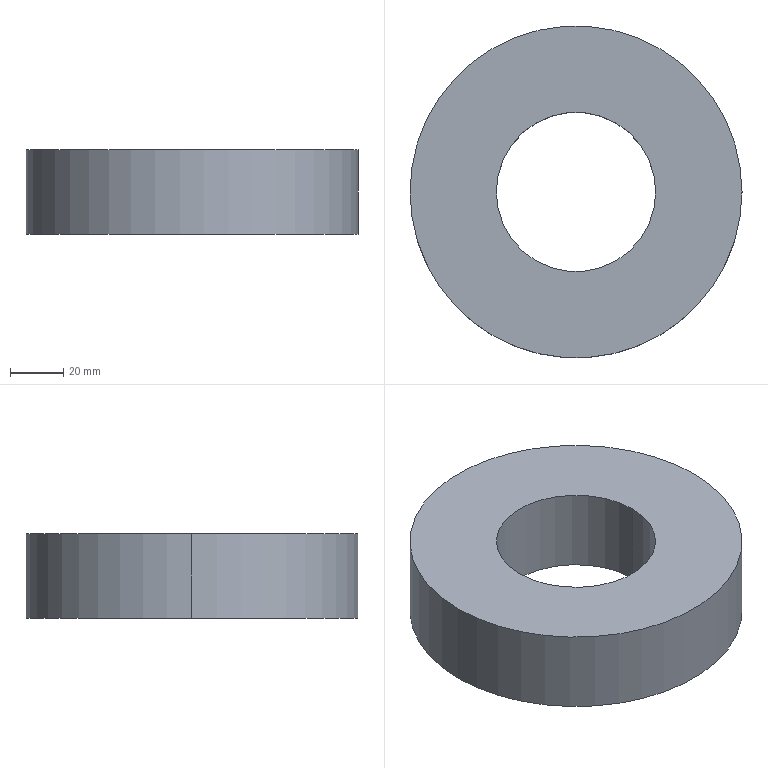Part | SolidWorks | features Extrusion 1 | 1 solid | 6 faces | box 125 x 125 x 32 mm | volume 302221 mm3 | cylinder 4 | plane 2 | commonest cylinder face diameters 60 x2 125 x2
STEP:
#1=CARTESIAN_POINT('',(-30.,0.,-16.));
#2=VERTEX_POINT('',#1);
#3=CARTESIAN_POINT('',(30.,0.,-16.));
#4=VERTEX_POINT('',#3);
#5=CARTESIAN_POINT('',(0.,0.,-16.));
#6=DIRECTION('',(0.,0.,1.));
#7=DIRECTION('',(1.,0.,0.));
#8=AXIS2_PLACEMENT_3D('',#5,#6,#7);
#9=CIRCLE('',#8,30.);
#10=EDGE_CURVE('',#2,#4,#9,.T.);
#11=ORIENTED_EDGE('',*,*,#10,.F.);
#12=CARTESIAN_POINT('',(-30.,0.,16.));
#13=VERTEX_POINT('',#12);
#14=CARTESIAN_POINT('',(-30.,0.,-16.));
#15=DIRECTION('',(0.,0.,1.));
#16=VECTOR('',#15,1000.);
#17=LINE('',#14,#16);
#18=EDGE_CURVE('',#2,#13,#17,.T.);
#19=ORIENTED_EDGE('',*,*,#18,.T.);
#20=CARTESIAN_POINT('',(30.,0.,16.));
#21=VERTEX_POINT('',#20);
#22=CARTESIAN_POINT('',(0.,0.,16.));
#23=DIRECTION('',(0.,0.,1.));
#24=DIRECTION('',(1.,0.,0.));
#25=AXIS2_PLACEMENT_3D('',#22,#23,#24);
#26=CIRCLE('',#25,30.);
#27=EDGE_CURVE('',#13,#21,#26,.T.);
#28=ORIENTED_EDGE('',*,*,#27,.T.);
#29=CARTESIAN_POINT('',(30.,0.,-16.));
#30=DIRECTION('',(0.,0.,1.));
#31=VECTOR('',#30,1000.);
#32=LINE('',#29,#31);
#33=EDGE_CURVE('',#4,#21,#32,.T.);
#34=ORIENTED_EDGE('',*,*,#33,.F.);
#35=EDGE_LOOP('',(#11,#19,#28,#34));
#36=FACE_OUTER_BOUND('',#35,.T.);
#37=CARTESIAN_POINT('',(0.,0.,-16.));
#38=DIRECTION('',(0.,0.,1.));
#39=DIRECTION('',(1.,0.,0.));
#40=AXIS2_PLACEMENT_3D('',#37,#38,#39);
#41=CYLINDRICAL_SURFACE('',#40,30.);
#42=ADVANCED_FACE('',(#36),#41,.F.);
#43=CARTESIAN_POINT('',(62.5,0.,-16.));
#44=VERTEX_POINT('',#43);
#45=CARTESIAN_POINT('',(-62.5,0.,-16.));
#46=VERTEX_POINT('',#45);
#47=CARTESIAN_POINT('',(0.,0.,-16.));
#48=DIRECTION('',(0.,0.,1.));
#49=DIRECTION('',(1.,0.,0.));
#50=AXIS2_PLACEMENT_3D('',#47,#48,#49);
#51=CIRCLE('',#50,62.5);
#52=EDGE_CURVE('',#44,#46,#51,.T.);
#53=ORIENTED_EDGE('',*,*,#52,.T.);
#54=CARTESIAN_POINT('',(-62.5,0.,16.));
#55=VERTEX_POINT('',#54);
#56=CARTESIAN_POINT('',(-62.5,0.,-16.));
#57=DIRECTION('',(0.,0.,1.));
#58=VECTOR('',#57,1000.);
#59=LINE('',#56,#58);
#60=EDGE_CURVE('',#46,#55,#59,.T.);
#61=ORIENTED_EDGE('',*,*,#60,.T.);
#62=CARTESIAN_POINT('',(62.5,0.,16.));
#63=VERTEX_POINT('',#62);
#64=CARTESIAN_POINT('',(0.,0.,16.));
#65=DIRECTION('',(0.,0.,1.));
#66=DIRECTION('',(1.,0.,0.));
#67=AXIS2_PLACEMENT_3D('',#64,#65,#66);
#68=CIRCLE('',#67,62.5);
#69=EDGE_CURVE('',#63,#55,#68,.T.);
#70=ORIENTED_EDGE('',*,*,#69,.F.);
#71=CARTESIAN_POINT('',(62.5,0.,-16.));
#72=DIRECTION('',(0.,0.,1.));
#73=VECTOR('',#72,1000.);
#74=LINE('',#71,#73);
#75=EDGE_CURVE('',#44,#63,#74,.T.);
#76=ORIENTED_EDGE('',*,*,#75,.F.);
#77=EDGE_LOOP('',(#53,#61,#70,#76));
#78=FACE_OUTER_BOUND('',#77,.T.);
#79=CARTESIAN_POINT('',(0.,0.,-16.));
#80=DIRECTION('',(0.,0.,1.));
#81=DIRECTION('',(1.,0.,0.));
#82=AXIS2_PLACEMENT_3D('',#79,#80,#81);
#83=CYLINDRICAL_SURFACE('',#82,62.5);
#84=ADVANCED_FACE('',(#78),#83,.T.);
#85=ORIENTED_EDGE('',*,*,#60,.F.);
#86=CARTESIAN_POINT('',(0.,0.,-16.));
#87=DIRECTION('',(0.,0.,1.));
#88=DIRECTION('',(1.,0.,0.));
#89=AXIS2_PLACEMENT_3D('',#86,#87,#88);
#90=CIRCLE('',#89,62.5);
#91=EDGE_CURVE('',#46,#44,#90,.T.);
#92=ORIENTED_EDGE('',*,*,#91,.T.);
#93=ORIENTED_EDGE('',*,*,#75,.T.);
#94=CARTESIAN_POINT('',(0.,0.,16.));
#95=DIRECTION('',(0.,0.,1.));
#96=DIRECTION('',(1.,0.,0.));
#97=AXIS2_PLACEMENT_3D('',#94,#95,#96);
#98=CIRCLE('',#97,62.5);
#99=EDGE_CURVE('',#55,#63,#98,.T.);
#100=ORIENTED_EDGE('',*,*,#99,.F.);
#101=EDGE_LOOP('',(#85,#92,#93,#100));
#102=FACE_OUTER_BOUND('',#101,.T.);
#103=CARTESIAN_POINT('',(0.,0.,-16.));
#104=DIRECTION('',(0.,0.,1.));
#105=DIRECTION('',(1.,0.,0.));
#106=AXIS2_PLACEMENT_3D('',#103,#104,#105);
#107=CYLINDRICAL_SURFACE('',#106,62.5);
#108=ADVANCED_FACE('',(#102),#107,.T.);
#109=CARTESIAN_POINT('',(0.,0.,-16.));
#110=DIRECTION('',(0.,0.,1.));
#111=DIRECTION('',(1.,0.,0.));
#112=AXIS2_PLACEMENT_3D('',#109,#110,#111);
#113=CIRCLE('',#112,30.);
#114=EDGE_CURVE('',#4,#2,#113,.T.);
#115=ORIENTED_EDGE('',*,*,#114,.T.);
#116=ORIENTED_EDGE('',*,*,#10,.T.);
#117=EDGE_LOOP('',(#115,#116));
#118=FACE_BOUND('',#117,.T.);
#119=ORIENTED_EDGE('',*,*,#52,.F.);
#120=ORIENTED_EDGE('',*,*,#91,.F.);
#121=EDGE_LOOP('',(#119,#120));
#122=FACE_OUTER_BOUND('',#121,.T.);
#123=CARTESIAN_POINT('',(0.,0.,-16.));
#124=DIRECTION('',(0.,0.,1.));
#125=DIRECTION('',(1.,0.,0.));
#126=AXIS2_PLACEMENT_3D('',#123,#124,#125);
#127=PLANE('',#126);
#128=ADVANCED_FACE('',(#118,#122),#127,.F.);
#129=CARTESIAN_POINT('',(0.,0.,16.));
#130=DIRECTION('',(0.,0.,1.));
#131=DIRECTION('',(1.,0.,0.));
#132=AXIS2_PLACEMENT_3D('',#129,#130,#131);
#133=CIRCLE('',#132,30.);
#134=EDGE_CURVE('',#21,#13,#133,.T.);
#135=ORIENTED_EDGE('',*,*,#134,.F.);
#136=ORIENTED_EDGE('',*,*,#27,.F.);
#137=EDGE_LOOP('',(#135,#136));
#138=FACE_BOUND('',#137,.T.);
#139=ORIENTED_EDGE('',*,*,#69,.T.);
#140=ORIENTED_EDGE('',*,*,#99,.T.);
#141=EDGE_LOOP('',(#139,#140));
#142=FACE_OUTER_BOUND('',#141,.T.);
#143=CARTESIAN_POINT('',(0.,0.,16.));
#144=DIRECTION('',(0.,0.,1.));
#145=DIRECTION('',(1.,0.,0.));
#146=AXIS2_PLACEMENT_3D('',#143,#144,#145);
#147=PLANE('',#146);
#148=ADVANCED_FACE('',(#138,#142),#147,.T.);
#149=ORIENTED_EDGE('',*,*,#18,.F.);
#150=ORIENTED_EDGE('',*,*,#114,.F.);
#151=ORIENTED_EDGE('',*,*,#33,.T.);
#152=ORIENTED_EDGE('',*,*,#134,.T.);
#153=EDGE_LOOP('',(#149,#150,#151,#152));
#154=FACE_OUTER_BOUND('',#153,.T.);
#155=CARTESIAN_POINT('',(0.,0.,-16.));
#156=DIRECTION('',(0.,0.,1.));
#157=DIRECTION('',(1.,0.,0.));
#158=AXIS2_PLACEMENT_3D('',#155,#156,#157);
#159=CYLINDRICAL_SURFACE('',#158,30.);
#160=ADVANCED_FACE('',(#154),#159,.F.);
#161=CLOSED_SHELL('',(#42,#84,#108,#128,#148,#160));
#162=MANIFOLD_SOLID_BREP('',#161);
#163=CARTESIAN_POINT('',(0.,0.,0.));
#164=DIRECTION('',(0.,0.,1.));
#165=DIRECTION('',(1.,0.,0.));
#166=AXIS2_PLACEMENT_3D('',#163,#164,#165);
#167=(LENGTH_UNIT()NAMED_UNIT(*)SI_UNIT(.MILLI.,.METRE.));
#168=UNCERTAINTY_MEASURE_WITH_UNIT(LENGTH_MEASURE(0.00001),#167,'','');
#169=(NAMED_UNIT(*)PLANE_ANGLE_UNIT()SI_UNIT($,.RADIAN.));
#170=(NAMED_UNIT(*)SI_UNIT($,.STERADIAN.)SOLID_ANGLE_UNIT());
#171=(GEOMETRIC_REPRESENTATION_CONTEXT(3)GLOBAL_UNCERTAINTY_ASSIGNED_CONTEXT((#168))GLOBAL_UNIT_ASSIGNED_CONTEXT((#167,#169,#170))REPRESENTATION_CONTEXT('',''));
#172=ADVANCED_BREP_SHAPE_REPRESENTATION('',(#162,#166),#171);